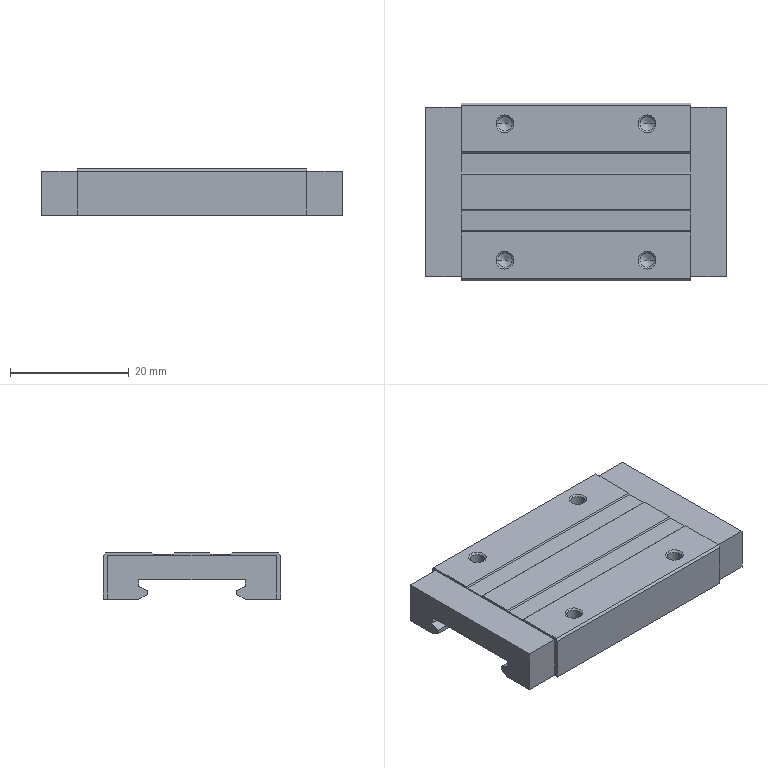Part | SolidWorks | features BaseBody 1 | 1 solid | 66 faces | box 50.7 x 30 x 7.8 mm | volume 8668 mm3 | plane 34 | cone 16 | cylinder 16 | commonest cylinder face diameters 2.449 x8 2.459 x8